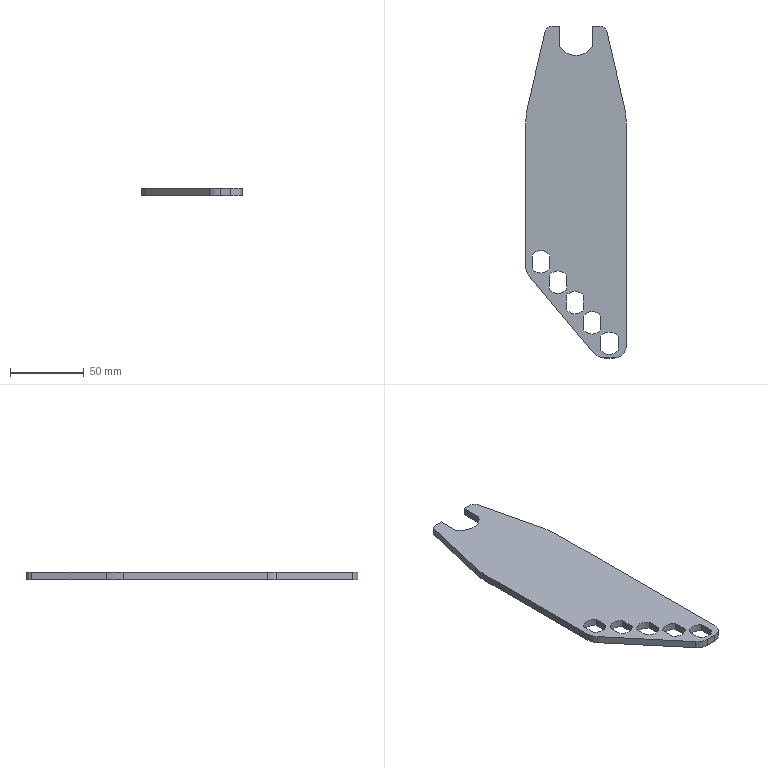Part | SolidWorks | features Fillet 5, ICE 5, Extrusion 1, LPattern 1 | 1 solid | 40 faces | box 68 x 225 x 5 mm | volume 59113 mm3 | plane 22 | cylinder 18 | commonest cylinder face diameters 15.2 x10 10 x2 20 x2 100 x2 16 x1 26 x1
STEP:
#1=CARTESIAN_POINT('',(-29.781,-52.01,5.));
#2=VERTEX_POINT('',#1);
#3=CARTESIAN_POINT('',(-17.781,-52.01,5.));
#4=VERTEX_POINT('',#3);
#5=CARTESIAN_POINT('',(-23.781,-47.345,5.));
#6=DIRECTION('',(0.,0.,1.));
#7=DIRECTION('',(1.,0.,0.));
#8=AXIS2_PLACEMENT_3D('',#5,#6,#7);
#9=CIRCLE('',#8,7.6);
#10=EDGE_CURVE('',#2,#4,#9,.T.);
#11=ORIENTED_EDGE('',*,*,#10,.T.);
#12=CARTESIAN_POINT('',(-17.781,-52.01,0.));
#13=VERTEX_POINT('',#12);
#14=CARTESIAN_POINT('',(-17.781,-52.01,0.));
#15=DIRECTION('',(0.,0.,1.));
#16=VECTOR('',#15,1000.);
#17=LINE('',#14,#16);
#18=EDGE_CURVE('',#13,#4,#17,.T.);
#19=ORIENTED_EDGE('',*,*,#18,.F.);
#20=CARTESIAN_POINT('',(-29.781,-52.01,0.));
#21=VERTEX_POINT('',#20);
#22=CARTESIAN_POINT('',(-23.781,-47.345,0.));
#23=DIRECTION('',(0.,0.,1.));
#24=DIRECTION('',(1.,0.,0.));
#25=AXIS2_PLACEMENT_3D('',#22,#23,#24);
#26=CIRCLE('',#25,7.6);
#27=EDGE_CURVE('',#21,#13,#26,.T.);
#28=ORIENTED_EDGE('',*,*,#27,.F.);
#29=CARTESIAN_POINT('',(-29.781,-52.01,0.));
#30=DIRECTION('',(0.,0.,1.));
#31=VECTOR('',#30,1000.);
#32=LINE('',#29,#31);
#33=EDGE_CURVE('',#21,#2,#32,.T.);
#34=ORIENTED_EDGE('',*,*,#33,.T.);
#35=EDGE_LOOP('',(#11,#19,#28,#34));
#36=FACE_OUTER_BOUND('',#35,.T.);
#37=CARTESIAN_POINT('',(-23.781,-47.345,-3.));
#38=DIRECTION('',(0.,0.,1.));
#39=DIRECTION('',(1.,0.,0.));
#40=AXIS2_PLACEMENT_3D('',#37,#38,#39);
#41=CYLINDRICAL_SURFACE('',#40,7.6);
#42=ADVANCED_FACE('',(#36),#41,.F.);
#43=CARTESIAN_POINT('',(-18.211,-65.798,5.));
#44=VERTEX_POINT('',#43);
#45=CARTESIAN_POINT('',(-6.211,-65.798,5.));
#46=VERTEX_POINT('',#45);
#47=CARTESIAN_POINT('',(-12.211,-61.134,5.));
#48=DIRECTION('',(0.,0.,1.));
#49=DIRECTION('',(1.,0.,0.));
#50=AXIS2_PLACEMENT_3D('',#47,#48,#49);
#51=CIRCLE('',#50,7.6);
#52=EDGE_CURVE('',#44,#46,#51,.T.);
#53=ORIENTED_EDGE('',*,*,#52,.T.);
#54=CARTESIAN_POINT('',(-6.211,-65.798,0.));
#55=VERTEX_POINT('',#54);
#56=CARTESIAN_POINT('',(-6.211,-65.798,0.));
#57=DIRECTION('',(0.,0.,1.));
#58=VECTOR('',#57,1000.);
#59=LINE('',#56,#58);
#60=EDGE_CURVE('',#55,#46,#59,.T.);
#61=ORIENTED_EDGE('',*,*,#60,.F.);
#62=CARTESIAN_POINT('',(-18.211,-65.798,0.));
#63=VERTEX_POINT('',#62);
#64=CARTESIAN_POINT('',(-12.211,-61.134,0.));
#65=DIRECTION('',(0.,0.,1.));
#66=DIRECTION('',(1.,0.,0.));
#67=AXIS2_PLACEMENT_3D('',#64,#65,#66);
#68=CIRCLE('',#67,7.6);
#69=EDGE_CURVE('',#63,#55,#68,.T.);
#70=ORIENTED_EDGE('',*,*,#69,.F.);
#71=CARTESIAN_POINT('',(-18.211,-65.798,0.));
#72=DIRECTION('',(0.,0.,1.));
#73=VECTOR('',#72,1000.);
#74=LINE('',#71,#73);
#75=EDGE_CURVE('',#63,#44,#74,.T.);
#76=ORIENTED_EDGE('',*,*,#75,.T.);
#77=EDGE_LOOP('',(#53,#61,#70,#76));
#78=FACE_OUTER_BOUND('',#77,.T.);
#79=CARTESIAN_POINT('',(-12.211,-61.134,-3.));
#80=DIRECTION('',(0.,0.,1.));
#81=DIRECTION('',(1.,0.,0.));
#82=AXIS2_PLACEMENT_3D('',#79,#80,#81);
#83=CYLINDRICAL_SURFACE('',#82,7.6);
#84=ADVANCED_FACE('',(#78),#83,.F.);
#85=CARTESIAN_POINT('',(-6.64,-79.587,5.));
#86=VERTEX_POINT('',#85);
#87=CARTESIAN_POINT('',(5.36,-79.587,5.));
#88=VERTEX_POINT('',#87);
#89=CARTESIAN_POINT('',(-0.6404,-74.922,5.));
#90=DIRECTION('',(0.,0.,1.));
#91=DIRECTION('',(1.,0.,0.));
#92=AXIS2_PLACEMENT_3D('',#89,#90,#91);
#93=CIRCLE('',#92,7.6);
#94=EDGE_CURVE('',#86,#88,#93,.T.);
#95=ORIENTED_EDGE('',*,*,#94,.T.);
#96=CARTESIAN_POINT('',(5.36,-79.587,0.));
#97=VERTEX_POINT('',#96);
#98=CARTESIAN_POINT('',(5.36,-79.587,0.));
#99=DIRECTION('',(0.,0.,1.));
#100=VECTOR('',#99,1000.);
#101=LINE('',#98,#100);
#102=EDGE_CURVE('',#97,#88,#101,.T.);
#103=ORIENTED_EDGE('',*,*,#102,.F.);
#104=CARTESIAN_POINT('',(-6.64,-79.587,0.));
#105=VERTEX_POINT('',#104);
#106=CARTESIAN_POINT('',(-0.6404,-74.922,0.));
#107=DIRECTION('',(0.,0.,1.));
#108=DIRECTION('',(1.,0.,0.));
#109=AXIS2_PLACEMENT_3D('',#106,#107,#108);
#110=CIRCLE('',#109,7.6);
#111=EDGE_CURVE('',#105,#97,#110,.T.);
#112=ORIENTED_EDGE('',*,*,#111,.F.);
#113=CARTESIAN_POINT('',(-6.64,-79.587,0.));
#114=DIRECTION('',(0.,0.,1.));
#115=VECTOR('',#114,1000.);
#116=LINE('',#113,#115);
#117=EDGE_CURVE('',#105,#86,#116,.T.);
#118=ORIENTED_EDGE('',*,*,#117,.T.);
#119=EDGE_LOOP('',(#95,#103,#112,#118));
#120=FACE_OUTER_BOUND('',#119,.T.);
#121=CARTESIAN_POINT('',(-0.6404,-74.922,-3.));
#122=DIRECTION('',(0.,0.,1.));
#123=DIRECTION('',(1.,0.,0.));
#124=AXIS2_PLACEMENT_3D('',#121,#122,#123);
#125=CYLINDRICAL_SURFACE('',#124,7.6);
#126=ADVANCED_FACE('',(#120),#125,.F.);
#127=CARTESIAN_POINT('',(4.93,-93.376,5.));
#128=VERTEX_POINT('',#127);
#129=CARTESIAN_POINT('',(16.93,-93.376,5.));
#130=VERTEX_POINT('',#129);
#131=CARTESIAN_POINT('',(10.93,-88.711,5.));
#132=DIRECTION('',(0.,0.,1.));
#133=DIRECTION('',(1.,0.,0.));
#134=AXIS2_PLACEMENT_3D('',#131,#132,#133);
#135=CIRCLE('',#134,7.6);
#136=EDGE_CURVE('',#128,#130,#135,.T.);
#137=ORIENTED_EDGE('',*,*,#136,.T.);
#138=CARTESIAN_POINT('',(16.93,-93.376,0.));
#139=VERTEX_POINT('',#138);
#140=CARTESIAN_POINT('',(16.93,-93.376,0.));
#141=DIRECTION('',(0.,0.,1.));
#142=VECTOR('',#141,1000.);
#143=LINE('',#140,#142);
#144=EDGE_CURVE('',#139,#130,#143,.T.);
#145=ORIENTED_EDGE('',*,*,#144,.F.);
#146=CARTESIAN_POINT('',(4.93,-93.376,0.));
#147=VERTEX_POINT('',#146);
#148=CARTESIAN_POINT('',(10.93,-88.711,0.));
#149=DIRECTION('',(0.,0.,1.));
#150=DIRECTION('',(1.,0.,0.));
#151=AXIS2_PLACEMENT_3D('',#148,#149,#150);
#152=CIRCLE('',#151,7.6);
#153=EDGE_CURVE('',#147,#139,#152,.T.);
#154=ORIENTED_EDGE('',*,*,#153,.F.);
#155=CARTESIAN_POINT('',(4.93,-93.376,0.));
#156=DIRECTION('',(0.,0.,1.));
#157=VECTOR('',#156,1000.);
#158=LINE('',#155,#157);
#159=EDGE_CURVE('',#147,#128,#158,.T.);
#160=ORIENTED_EDGE('',*,*,#159,.T.);
#161=EDGE_LOOP('',(#137,#145,#154,#160));
#162=FACE_OUTER_BOUND('',#161,.T.);
#163=CARTESIAN_POINT('',(10.93,-88.711,-3.));
#164=DIRECTION('',(0.,0.,1.));
#165=DIRECTION('',(1.,0.,0.));
#166=AXIS2_PLACEMENT_3D('',#163,#164,#165);
#167=CYLINDRICAL_SURFACE('',#166,7.6);
#168=ADVANCED_FACE('',(#162),#167,.F.);
#169=CARTESIAN_POINT('',(16.5,-107.165,5.));
#170=VERTEX_POINT('',#169);
#171=CARTESIAN_POINT('',(28.5,-107.165,5.));
#172=VERTEX_POINT('',#171);
#173=CARTESIAN_POINT('',(22.5,-102.5,5.));
#174=DIRECTION('',(0.,0.,1.));
#175=DIRECTION('',(1.,0.,0.));
#176=AXIS2_PLACEMENT_3D('',#173,#174,#175);
#177=CIRCLE('',#176,7.6);
#178=EDGE_CURVE('',#170,#172,#177,.T.);
#179=ORIENTED_EDGE('',*,*,#178,.T.);
#180=CARTESIAN_POINT('',(28.5,-107.165,0.));
#181=VERTEX_POINT('',#180);
#182=CARTESIAN_POINT('',(28.5,-107.165,0.));
#183=DIRECTION('',(0.,0.,1.));
#184=VECTOR('',#183,1000.);
#185=LINE('',#182,#184);
#186=EDGE_CURVE('',#181,#172,#185,.T.);
#187=ORIENTED_EDGE('',*,*,#186,.F.);
#188=CARTESIAN_POINT('',(16.5,-107.165,0.));
#189=VERTEX_POINT('',#188);
#190=CARTESIAN_POINT('',(22.5,-102.5,0.));
#191=DIRECTION('',(0.,0.,1.));
#192=DIRECTION('',(1.,0.,0.));
#193=AXIS2_PLACEMENT_3D('',#190,#191,#192);
#194=CIRCLE('',#193,7.6);
#195=EDGE_CURVE('',#189,#181,#194,.T.);
#196=ORIENTED_EDGE('',*,*,#195,.F.);
#197=CARTESIAN_POINT('',(16.5,-107.165,0.));
#198=DIRECTION('',(0.,0.,1.));
#199=VECTOR('',#198,1000.);
#200=LINE('',#197,#199);
#201=EDGE_CURVE('',#189,#170,#200,.T.);
#202=ORIENTED_EDGE('',*,*,#201,.T.);
#203=EDGE_LOOP('',(#179,#187,#196,#202));
#204=FACE_OUTER_BOUND('',#203,.T.);
#205=CARTESIAN_POINT('',(22.5,-102.5,-3.));
#206=DIRECTION('',(0.,0.,1.));
#207=DIRECTION('',(1.,0.,0.));
#208=AXIS2_PLACEMENT_3D('',#205,#206,#207);
#209=CYLINDRICAL_SURFACE('',#208,7.6);
#210=ADVANCED_FACE('',(#204),#209,.F.);
#211=CARTESIAN_POINT('',(16.032,112.5,5.));
#212=VERTEX_POINT('',#211);
#213=CARTESIAN_POINT('',(11.,112.5,5.));
#214=VERTEX_POINT('',#213);
#215=CARTESIAN_POINT('',(-34.,112.5,5.));
#216=DIRECTION('',(-1.,0.,0.));
#217=VECTOR('',#216,1000.);
#218=LINE('',#215,#217);
#219=EDGE_CURVE('',#212,#214,#218,.T.);
#220=ORIENTED_EDGE('',*,*,#219,.F.);
#221=CARTESIAN_POINT('',(16.032,112.5,0.));
#222=VERTEX_POINT('',#221);
#223=CARTESIAN_POINT('',(16.032,112.5,5.));
#224=DIRECTION('',(0.,0.,-1.));
#225=VECTOR('',#224,1000.);
#226=LINE('',#223,#225);
#227=EDGE_CURVE('',#212,#222,#226,.T.);
#228=ORIENTED_EDGE('',*,*,#227,.T.);
#229=CARTESIAN_POINT('',(11.,112.5,0.));
#230=VERTEX_POINT('',#229);
#231=CARTESIAN_POINT('',(-34.,112.5,0.));
#232=DIRECTION('',(-1.,0.,0.));
#233=VECTOR('',#232,1000.);
#234=LINE('',#231,#233);
#235=EDGE_CURVE('',#222,#230,#234,.T.);
#236=ORIENTED_EDGE('',*,*,#235,.T.);
#237=CARTESIAN_POINT('',(11.,112.5,-3.));
#238=DIRECTION('',(0.,0.,1.));
#239=VECTOR('',#238,1000.);
#240=LINE('',#237,#239);
#241=EDGE_CURVE('',#230,#214,#240,.T.);
#242=ORIENTED_EDGE('',*,*,#241,.T.);
#243=EDGE_LOOP('',(#220,#228,#236,#242));
#244=FACE_OUTER_BOUND('',#243,.T.);
#245=CARTESIAN_POINT('',(-34.,112.5,5.));
#246=DIRECTION('',(0.,-1.,0.));
#247=DIRECTION('',(0.,0.,-1.));
#248=AXIS2_PLACEMENT_3D('',#245,#246,#247);
#249=PLANE('',#248);
#250=ADVANCED_FACE('',(#244),#249,.F.);
#251=CARTESIAN_POINT('',(34.,-104.5,0.));
#252=VERTEX_POINT('',#251);
#253=CARTESIAN_POINT('',(34.,46.744,0.));
#254=VERTEX_POINT('',#253);
#255=CARTESIAN_POINT('',(34.,112.5,0.));
#256=DIRECTION('',(0.,1.,0.));
#257=VECTOR('',#256,1000.);
#258=LINE('',#255,#257);
#259=EDGE_CURVE('',#252,#254,#258,.T.);
#260=ORIENTED_EDGE('',*,*,#259,.T.);
#261=CARTESIAN_POINT('',(34.,46.744,5.));
#262=VERTEX_POINT('',#261);
#263=CARTESIAN_POINT('',(34.,46.744,5.));
#264=DIRECTION('',(0.,0.,1.));
#265=VECTOR('',#264,1000.);
#266=LINE('',#263,#265);
#267=EDGE_CURVE('',#254,#262,#266,.T.);
#268=ORIENTED_EDGE('',*,*,#267,.T.);
#269=CARTESIAN_POINT('',(34.,-104.5,5.));
#270=VERTEX_POINT('',#269);
#271=CARTESIAN_POINT('',(34.,112.5,5.));
#272=DIRECTION('',(0.,1.,0.));
#273=VECTOR('',#272,1000.);
#274=LINE('',#271,#273);
#275=EDGE_CURVE('',#270,#262,#274,.T.);
#276=ORIENTED_EDGE('',*,*,#275,.F.);
#277=CARTESIAN_POINT('',(34.,-104.5,5.));
#278=DIRECTION('',(0.,0.,-1.));
#279=VECTOR('',#278,1000.);
#280=LINE('',#277,#279);
#281=EDGE_CURVE('',#270,#252,#280,.T.);
#282=ORIENTED_EDGE('',*,*,#281,.T.);
#283=EDGE_LOOP('',(#260,#268,#276,#282));
#284=FACE_OUTER_BOUND('',#283,.T.);
#285=CARTESIAN_POINT('',(34.,112.5,5.));
#286=DIRECTION('',(-1.,0.,0.));
#287=DIRECTION('',(0.,-1.,0.));
#288=AXIS2_PLACEMENT_3D('',#285,#286,#287);
#289=PLANE('',#288);
#290=ADVANCED_FACE('',(#284),#289,.F.);
#291=CARTESIAN_POINT('',(-11.,112.5,0.));
#292=VERTEX_POINT('',#291);
#293=CARTESIAN_POINT('',(-16.032,112.5,0.));
#294=VERTEX_POINT('',#293);
#295=CARTESIAN_POINT('',(-34.,112.5,0.));
#296=DIRECTION('',(-1.,0.,0.));
#297=VECTOR('',#296,1000.);
#298=LINE('',#295,#297);
#299=EDGE_CURVE('',#292,#294,#298,.T.);
#300=ORIENTED_EDGE('',*,*,#299,.T.);
#301=CARTESIAN_POINT('',(-16.032,112.5,5.));
#302=VERTEX_POINT('',#301);
#303=CARTESIAN_POINT('',(-16.032,112.5,5.));
#304=DIRECTION('',(0.,0.,1.));
#305=VECTOR('',#304,1000.);
#306=LINE('',#303,#305);
#307=EDGE_CURVE('',#294,#302,#306,.T.);
#308=ORIENTED_EDGE('',*,*,#307,.T.);
#309=CARTESIAN_POINT('',(-11.,112.5,5.));
#310=VERTEX_POINT('',#309);
#311=CARTESIAN_POINT('',(-34.,112.5,5.));
#312=DIRECTION('',(-1.,0.,0.));
#313=VECTOR('',#312,1000.);
#314=LINE('',#311,#313);
#315=EDGE_CURVE('',#310,#302,#314,.T.);
#316=ORIENTED_EDGE('',*,*,#315,.F.);
#317=CARTESIAN_POINT('',(-11.,112.5,-3.));
#318=DIRECTION('',(0.,0.,1.));
#319=VECTOR('',#318,1000.);
#320=LINE('',#317,#319);
#321=EDGE_CURVE('',#292,#310,#320,.T.);
#322=ORIENTED_EDGE('',*,*,#321,.F.);
#323=EDGE_LOOP('',(#300,#308,#316,#322));
#324=FACE_OUTER_BOUND('',#323,.T.);
#325=CARTESIAN_POINT('',(-34.,112.5,5.));
#326=DIRECTION('',(0.,-1.,0.));
#327=DIRECTION('',(0.,0.,-1.));
#328=AXIS2_PLACEMENT_3D('',#325,#326,#327);
#329=PLANE('',#328);
#330=ADVANCED_FACE('',(#324),#329,.F.);
#331=CARTESIAN_POINT('',(-34.,46.744,5.));
#332=VERTEX_POINT('',#331);
#333=CARTESIAN_POINT('',(-34.,-50.973,5.));
#334=VERTEX_POINT('',#333);
#335=CARTESIAN_POINT('',(-34.,112.5,5.));
#336=DIRECTION('',(0.,-1.,0.));
#337=VECTOR('',#336,1000.);
#338=LINE('',#335,#337);
#339=EDGE_CURVE('',#332,#334,#338,.T.);
#340=ORIENTED_EDGE('',*,*,#339,.F.);
#341=CARTESIAN_POINT('',(-34.,46.744,0.));
#342=VERTEX_POINT('',#341);
#343=CARTESIAN_POINT('',(-34.,46.744,5.));
#344=DIRECTION('',(0.,0.,-1.));
#345=VECTOR('',#344,1000.);
#346=LINE('',#343,#345);
#347=EDGE_CURVE('',#332,#342,#346,.T.);
#348=ORIENTED_EDGE('',*,*,#347,.T.);
#349=CARTESIAN_POINT('',(-34.,-50.973,0.));
#350=VERTEX_POINT('',#349);
#351=CARTESIAN_POINT('',(-34.,112.5,0.));
#352=DIRECTION('',(0.,-1.,0.));
#353=VECTOR('',#352,1000.);
#354=LINE('',#351,#353);
#355=EDGE_CURVE('',#342,#350,#354,.T.);
#356=ORIENTED_EDGE('',*,*,#355,.T.);
#357=CARTESIAN_POINT('',(-34.,-50.973,5.));
#358=DIRECTION('',(0.,0.,1.));
#359=VECTOR('',#358,1000.);
#360=LINE('',#357,#359);
#361=EDGE_CURVE('',#350,#334,#360,.T.);
#362=ORIENTED_EDGE('',*,*,#361,.T.);
#363=EDGE_LOOP('',(#340,#348,#356,#362));
#364=FACE_OUTER_BOUND('',#363,.T.);
#365=CARTESIAN_POINT('',(-34.,112.5,5.));
#366=DIRECTION('',(1.,0.,0.));
#367=DIRECTION('',(0.,1.,0.));
#368=AXIS2_PLACEMENT_3D('',#365,#366,#367);
#369=PLANE('',#368);
#370=ADVANCED_FACE('',(#364),#369,.F.);
#371=CARTESIAN_POINT('',(19.236,-112.5,5.));
#372=VERTEX_POINT('',#371);
#373=CARTESIAN_POINT('',(26.,-112.5,5.));
#374=VERTEX_POINT('',#373);
#375=CARTESIAN_POINT('',(-34.,-112.5,5.));
#376=DIRECTION('',(1.,0.,0.));
#377=VECTOR('',#376,1000.);
#378=LINE('',#375,#377);
#379=EDGE_CURVE('',#372,#374,#378,.T.);
#380=ORIENTED_EDGE('',*,*,#379,.F.);
#381=CARTESIAN_POINT('',(19.236,-112.5,0.));
#382=VERTEX_POINT('',#381);
#383=CARTESIAN_POINT('',(19.236,-112.5,5.));
#384=DIRECTION('',(0.,0.,-1.));
#385=VECTOR('',#384,1000.);
#386=LINE('',#383,#385);
#387=EDGE_CURVE('',#372,#382,#386,.T.);
#388=ORIENTED_EDGE('',*,*,#387,.T.);
#389=CARTESIAN_POINT('',(26.,-112.5,0.));
#390=VERTEX_POINT('',#389);
#391=CARTESIAN_POINT('',(-34.,-112.5,0.));
#392=DIRECTION('',(1.,0.,0.));
#393=VECTOR('',#392,1000.);
#394=LINE('',#391,#393);
#395=EDGE_CURVE('',#382,#390,#394,.T.);
#396=ORIENTED_EDGE('',*,*,#395,.T.);
#397=CARTESIAN_POINT('',(26.,-112.5,5.));
#398=DIRECTION('',(0.,0.,1.));
#399=VECTOR('',#398,1000.);
#400=LINE('',#397,#399);
#401=EDGE_CURVE('',#390,#374,#400,.T.);
#402=ORIENTED_EDGE('',*,*,#401,.T.);
#403=EDGE_LOOP('',(#380,#388,#396,#402));
#404=FACE_OUTER_BOUND('',#403,.T.);
#405=CARTESIAN_POINT('',(-34.,-112.5,5.));
#406=DIRECTION('',(0.,1.,0.));
#407=DIRECTION('',(0.,0.,1.));
#408=AXIS2_PLACEMENT_3D('',#405,#406,#407);
#409=PLANE('',#408);
#410=ADVANCED_FACE('',(#404),#409,.F.);
#411=ORIENTED_EDGE('',*,*,#275,.T.);
#412=CARTESIAN_POINT('',(32.692,58.105,5.));
#413=VERTEX_POINT('',#412);
#414=CARTESIAN_POINT('',(-16.,46.744,5.));
#415=DIRECTION('',(0.,0.,1.));
#416=DIRECTION('',(1.,0.,0.));
#417=AXIS2_PLACEMENT_3D('',#414,#415,#416);
#418=CIRCLE('',#417,50.);
#419=EDGE_CURVE('',#262,#413,#418,.T.);
#420=ORIENTED_EDGE('',*,*,#419,.T.);
#421=CARTESIAN_POINT('',(20.902,108.636,5.));
#422=VERTEX_POINT('',#421);
#423=CARTESIAN_POINT('',(20.,112.5,5.));
#424=DIRECTION('',(0.2272,-0.9738,0.));
#425=VECTOR('',#424,1000.);
#426=LINE('',#423,#425);
#427=EDGE_CURVE('',#422,#413,#426,.T.);
#428=ORIENTED_EDGE('',*,*,#427,.F.);
#429=CARTESIAN_POINT('',(16.032,107.5,5.));
#430=DIRECTION('',(0.,0.,1.));
#431=DIRECTION('',(1.,0.,0.));
#432=AXIS2_PLACEMENT_3D('',#429,#430,#431);
#433=CIRCLE('',#432,5.);
#434=EDGE_CURVE('',#422,#212,#433,.T.);
#435=ORIENTED_EDGE('',*,*,#434,.T.);
#436=ORIENTED_EDGE('',*,*,#219,.T.);
#437=CARTESIAN_POINT('',(11.,98.644,5.));
#438=VERTEX_POINT('',#437);
#439=CARTESIAN_POINT('',(11.,112.5,5.));
#440=DIRECTION('',(0.,1.,0.));
#441=VECTOR('',#440,1000.);
#442=LINE('',#439,#441);
#443=EDGE_CURVE('',#438,#214,#442,.T.);
#444=ORIENTED_EDGE('',*,*,#443,.F.);
#445=CARTESIAN_POINT('',(-11.,98.644,5.));
#446=VERTEX_POINT('',#445);
#447=CARTESIAN_POINT('',(0.,105.572,5.));
#448=DIRECTION('',(0.,0.,1.));
#449=DIRECTION('',(1.,0.,0.));
#450=AXIS2_PLACEMENT_3D('',#447,#448,#449);
#451=CIRCLE('',#450,13.);
#452=EDGE_CURVE('',#446,#438,#451,.T.);
#453=ORIENTED_EDGE('',*,*,#452,.F.);
#454=CARTESIAN_POINT('',(-11.,112.5,5.));
#455=DIRECTION('',(0.,-1.,0.));
#456=VECTOR('',#455,1000.);
#457=LINE('',#454,#456);
#458=EDGE_CURVE('',#310,#446,#457,.T.);
#459=ORIENTED_EDGE('',*,*,#458,.F.);
#460=ORIENTED_EDGE('',*,*,#315,.T.);
#461=CARTESIAN_POINT('',(-20.902,108.636,5.));
#462=VERTEX_POINT('',#461);
#463=CARTESIAN_POINT('',(-16.032,107.5,5.));
#464=DIRECTION('',(0.,0.,1.));
#465=DIRECTION('',(1.,0.,0.));
#466=AXIS2_PLACEMENT_3D('',#463,#464,#465);
#467=CIRCLE('',#466,5.);
#468=EDGE_CURVE('',#302,#462,#467,.T.);
#469=ORIENTED_EDGE('',*,*,#468,.T.);
#470=CARTESIAN_POINT('',(-32.692,58.105,5.));
#471=VERTEX_POINT('',#470);
#472=CARTESIAN_POINT('',(-20.,112.5,5.));
#473=DIRECTION('',(0.2272,0.9738,0.));
#474=VECTOR('',#473,1000.);
#475=LINE('',#472,#474);
#476=EDGE_CURVE('',#471,#462,#475,.T.);
#477=ORIENTED_EDGE('',*,*,#476,.F.);
#478=CARTESIAN_POINT('',(16.,46.744,5.));
#479=DIRECTION('',(0.,0.,1.));
#480=DIRECTION('',(1.,0.,0.));
#481=AXIS2_PLACEMENT_3D('',#478,#479,#480);
#482=CIRCLE('',#481,50.);
#483=EDGE_CURVE('',#471,#332,#482,.T.);
#484=ORIENTED_EDGE('',*,*,#483,.T.);
#485=ORIENTED_EDGE('',*,*,#339,.T.);
#486=CARTESIAN_POINT('',(-31.66,-57.401,5.));
#487=VERTEX_POINT('',#486);
#488=CARTESIAN_POINT('',(-24.,-50.973,5.));
#489=DIRECTION('',(0.,0.,1.));
#490=DIRECTION('',(1.,0.,0.));
#491=AXIS2_PLACEMENT_3D('',#488,#489,#490);
#492=CIRCLE('',#491,10.);
#493=EDGE_CURVE('',#334,#487,#492,.T.);
#494=ORIENTED_EDGE('',*,*,#493,.T.);
#495=CARTESIAN_POINT('',(11.576,-108.928,5.));
#496=VERTEX_POINT('',#495);
#497=CARTESIAN_POINT('',(14.573,-112.5,5.));
#498=DIRECTION('',(-0.6428,0.766,0.));
#499=VECTOR('',#498,1000.);
#500=LINE('',#497,#499);
#501=EDGE_CURVE('',#496,#487,#500,.T.);
#502=ORIENTED_EDGE('',*,*,#501,.F.);
#503=CARTESIAN_POINT('',(19.236,-102.5,5.));
#504=DIRECTION('',(0.,0.,1.));
#505=DIRECTION('',(1.,0.,0.));
#506=AXIS2_PLACEMENT_3D('',#503,#504,#505);
#507=CIRCLE('',#506,10.);
#508=EDGE_CURVE('',#496,#372,#507,.T.);
#509=ORIENTED_EDGE('',*,*,#508,.T.);
#510=ORIENTED_EDGE('',*,*,#379,.T.);
#511=CARTESIAN_POINT('',(26.,-104.5,5.));
#512=DIRECTION('',(0.,0.,1.));
#513=DIRECTION('',(1.,0.,0.));
#514=AXIS2_PLACEMENT_3D('',#511,#512,#513);
#515=CIRCLE('',#514,8.);
#516=EDGE_CURVE('',#374,#270,#515,.T.);
#517=ORIENTED_EDGE('',*,*,#516,.T.);
#518=EDGE_LOOP('',(#411,#420,#428,#435,#436,#444,#453,#459,#460,#469,#477,#484,#485,#494,#502,#509,#510,#517));
#519=FACE_OUTER_BOUND('',#518,.T.);
#520=ORIENTED_EDGE('',*,*,#94,.F.);
#521=CARTESIAN_POINT('',(-6.64,-70.258,5.));
#522=VERTEX_POINT('',#521);
#523=CARTESIAN_POINT('',(-6.64,-79.587,5.));
#524=DIRECTION('',(0.,1.,0.));
#525=VECTOR('',#524,1000.);
#526=LINE('',#523,#525);
#527=EDGE_CURVE('',#86,#522,#526,.T.);
#528=ORIENTED_EDGE('',*,*,#527,.T.);
#529=CARTESIAN_POINT('',(5.36,-70.258,5.));
#530=VERTEX_POINT('',#529);
#531=CARTESIAN_POINT('',(-0.6404,-74.922,5.));
#532=DIRECTION('',(0.,0.,1.));
#533=DIRECTION('',(1.,0.,0.));
#534=AXIS2_PLACEMENT_3D('',#531,#532,#533);
#535=CIRCLE('',#534,7.6);
#536=EDGE_CURVE('',#530,#522,#535,.T.);
#537=ORIENTED_EDGE('',*,*,#536,.F.);
#538=CARTESIAN_POINT('',(5.36,-79.587,5.));
#539=DIRECTION('',(0.,-1.,0.));
#540=VECTOR('',#539,1000.);
#541=LINE('',#538,#540);
#542=EDGE_CURVE('',#530,#88,#541,.T.);
#543=ORIENTED_EDGE('',*,*,#542,.T.);
#544=EDGE_LOOP('',(#520,#528,#537,#543));
#545=FACE_BOUND('',#544,.T.);
#546=ORIENTED_EDGE('',*,*,#136,.F.);
#547=CARTESIAN_POINT('',(4.93,-84.046,5.));
#548=VERTEX_POINT('',#547);
#549=CARTESIAN_POINT('',(4.93,-93.376,5.));
#550=DIRECTION('',(0.,1.,0.));
#551=VECTOR('',#550,1000.);
#552=LINE('',#549,#551);
#553=EDGE_CURVE('',#128,#548,#552,.T.);
#554=ORIENTED_EDGE('',*,*,#553,.T.);
#555=CARTESIAN_POINT('',(16.93,-84.046,5.));
#556=VERTEX_POINT('',#555);
#557=CARTESIAN_POINT('',(10.93,-88.711,5.));
#558=DIRECTION('',(0.,0.,1.));
#559=DIRECTION('',(1.,0.,0.));
#560=AXIS2_PLACEMENT_3D('',#557,#558,#559);
#561=CIRCLE('',#560,7.6);
#562=EDGE_CURVE('',#556,#548,#561,.T.);
#563=ORIENTED_EDGE('',*,*,#562,.F.);
#564=CARTESIAN_POINT('',(16.93,-93.376,5.));
#565=DIRECTION('',(0.,-1.,0.));
#566=VECTOR('',#565,1000.);
#567=LINE('',#564,#566);
#568=EDGE_CURVE('',#556,#130,#567,.T.);
#569=ORIENTED_EDGE('',*,*,#568,.T.);
#570=EDGE_LOOP('',(#546,#554,#563,#569));
#571=FACE_BOUND('',#570,.T.);
#572=ORIENTED_EDGE('',*,*,#10,.F.);
#573=CARTESIAN_POINT('',(-29.781,-42.68,5.));
#574=VERTEX_POINT('',#573);
#575=CARTESIAN_POINT('',(-29.781,-52.01,5.));
#576=DIRECTION('',(0.,1.,0.));
#577=VECTOR('',#576,1000.);
#578=LINE('',#575,#577);
#579=EDGE_CURVE('',#2,#574,#578,.T.);
#580=ORIENTED_EDGE('',*,*,#579,.T.);
#581=CARTESIAN_POINT('',(-17.781,-42.68,5.));
#582=VERTEX_POINT('',#581);
#583=CARTESIAN_POINT('',(-23.781,-47.345,5.));
#584=DIRECTION('',(0.,0.,1.));
#585=DIRECTION('',(1.,0.,0.));
#586=AXIS2_PLACEMENT_3D('',#583,#584,#585);
#587=CIRCLE('',#586,7.6);
#588=EDGE_CURVE('',#582,#574,#587,.T.);
#589=ORIENTED_EDGE('',*,*,#588,.F.);
#590=CARTESIAN_POINT('',(-17.781,-52.01,5.));
#591=DIRECTION('',(0.,-1.,0.));
#592=VECTOR('',#591,1000.);
#593=LINE('',#590,#592);
#594=EDGE_CURVE('',#582,#4,#593,.T.);
#595=ORIENTED_EDGE('',*,*,#594,.T.);
#596=EDGE_LOOP('',(#572,#580,#589,#595));
#597=FACE_BOUND('',#596,.T.);
#598=ORIENTED_EDGE('',*,*,#52,.F.);
#599=CARTESIAN_POINT('',(-18.211,-56.469,5.));
#600=VERTEX_POINT('',#599);
#601=CARTESIAN_POINT('',(-18.211,-65.798,5.));
#602=DIRECTION('',(0.,1.,0.));
#603=VECTOR('',#602,1000.);
#604=LINE('',#601,#603);
#605=EDGE_CURVE('',#44,#600,#604,.T.);
#606=ORIENTED_EDGE('',*,*,#605,.T.);
#607=CARTESIAN_POINT('',(-6.211,-56.469,5.));
#608=VERTEX_POINT('',#607);
#609=CARTESIAN_POINT('',(-12.211,-61.134,5.));
#610=DIRECTION('',(0.,0.,1.));
#611=DIRECTION('',(1.,0.,0.));
#612=AXIS2_PLACEMENT_3D('',#609,#610,#611);
#613=CIRCLE('',#612,7.6);
#614=EDGE_CURVE('',#608,#600,#613,.T.);
#615=ORIENTED_EDGE('',*,*,#614,.F.);
#616=CARTESIAN_POINT('',(-6.211,-65.798,5.));
#617=DIRECTION('',(0.,-1.,0.));
#618=VECTOR('',#617,1000.);
#619=LINE('',#616,#618);
#620=EDGE_CURVE('',#608,#46,#619,.T.);
#621=ORIENTED_EDGE('',*,*,#620,.T.);
#622=EDGE_LOOP('',(#598,#606,#615,#621));
#623=FACE_BOUND('',#622,.T.);
#624=ORIENTED_EDGE('',*,*,#178,.F.);
#625=CARTESIAN_POINT('',(16.5,-97.835,5.));
#626=VERTEX_POINT('',#625);
#627=CARTESIAN_POINT('',(16.5,-107.165,5.));
#628=DIRECTION('',(0.,1.,0.));
#629=VECTOR('',#628,1000.);
#630=LINE('',#627,#629);
#631=EDGE_CURVE('',#170,#626,#630,.T.);
#632=ORIENTED_EDGE('',*,*,#631,.T.);
#633=CARTESIAN_POINT('',(28.5,-97.835,5.));
#634=VERTEX_POINT('',#633);
#635=CARTESIAN_POINT('',(22.5,-102.5,5.));
#636=DIRECTION('',(0.,0.,1.));
#637=DIRECTION('',(1.,0.,0.));
#638=AXIS2_PLACEMENT_3D('',#635,#636,#637);
#639=CIRCLE('',#638,7.6);
#640=EDGE_CURVE('',#634,#626,#639,.T.);
#641=ORIENTED_EDGE('',*,*,#640,.F.);
#642=CARTESIAN_POINT('',(28.5,-107.165,5.));
#643=DIRECTION('',(0.,-1.,0.));
#644=VECTOR('',#643,1000.);
#645=LINE('',#642,#644);
#646=EDGE_CURVE('',#634,#172,#645,.T.);
#647=ORIENTED_EDGE('',*,*,#646,.T.);
#648=EDGE_LOOP('',(#624,#632,#641,#647));
#649=FACE_BOUND('',#648,.T.);
#650=CARTESIAN_POINT('',(0.,0.,5.));
#651=DIRECTION('',(0.,0.,1.));
#652=DIRECTION('',(1.,0.,0.));
#653=AXIS2_PLACEMENT_3D('',#650,#651,#652);
#654=PLANE('',#653);
#655=ADVANCED_FACE('',(#519,#545,#571,#597,#623,#649),#654,.T.);
#656=ORIENTED_EDGE('',*,*,#111,.T.);
#657=CARTESIAN_POINT('',(5.36,-70.258,0.));
#658=VERTEX_POINT('',#657);
#659=CARTESIAN_POINT('',(5.36,-79.587,0.));
#660=DIRECTION('',(0.,-1.,0.));
#661=VECTOR('',#660,1000.);
#662=LINE('',#659,#661);
#663=EDGE_CURVE('',#658,#97,#662,.T.);
#664=ORIENTED_EDGE('',*,*,#663,.F.);
#665=CARTESIAN_POINT('',(-6.64,-70.258,0.));
#666=VERTEX_POINT('',#665);
#667=CARTESIAN_POINT('',(-0.6404,-74.922,0.));
#668=DIRECTION('',(0.,0.,1.));
#669=DIRECTION('',(1.,0.,0.));
#670=AXIS2_PLACEMENT_3D('',#667,#668,#669);
#671=CIRCLE('',#670,7.6);
#672=EDGE_CURVE('',#658,#666,#671,.T.);
#673=ORIENTED_EDGE('',*,*,#672,.T.);
#674=CARTESIAN_POINT('',(-6.64,-79.587,0.));
#675=DIRECTION('',(0.,1.,0.));
#676=VECTOR('',#675,1000.);
#677=LINE('',#674,#676);
#678=EDGE_CURVE('',#105,#666,#677,.T.);
#679=ORIENTED_EDGE('',*,*,#678,.F.);
#680=EDGE_LOOP('',(#656,#664,#673,#679));
#681=FACE_BOUND('',#680,.T.);
#682=ORIENTED_EDGE('',*,*,#153,.T.);
#683=CARTESIAN_POINT('',(16.93,-84.046,0.));
#684=VERTEX_POINT('',#683);
#685=CARTESIAN_POINT('',(16.93,-93.376,0.));
#686=DIRECTION('',(0.,-1.,0.));
#687=VECTOR('',#686,1000.);
#688=LINE('',#685,#687);
#689=EDGE_CURVE('',#684,#139,#688,.T.);
#690=ORIENTED_EDGE('',*,*,#689,.F.);
#691=CARTESIAN_POINT('',(4.93,-84.046,0.));
#692=VERTEX_POINT('',#691);
#693=CARTESIAN_POINT('',(10.93,-88.711,0.));
#694=DIRECTION('',(0.,0.,1.));
#695=DIRECTION('',(1.,0.,0.));
#696=AXIS2_PLACEMENT_3D('',#693,#694,#695);
#697=CIRCLE('',#696,7.6);
#698=EDGE_CURVE('',#684,#692,#697,.T.);
#699=ORIENTED_EDGE('',*,*,#698,.T.);
#700=CARTESIAN_POINT('',(4.93,-93.376,0.));
#701=DIRECTION('',(0.,1.,0.));
#702=VECTOR('',#701,1000.);
#703=LINE('',#700,#702);
#704=EDGE_CURVE('',#147,#692,#703,.T.);
#705=ORIENTED_EDGE('',*,*,#704,.F.);
#706=EDGE_LOOP('',(#682,#690,#699,#705));
#707=FACE_BOUND('',#706,.T.);
#708=ORIENTED_EDGE('',*,*,#27,.T.);
#709=CARTESIAN_POINT('',(-17.781,-42.68,0.));
#710=VERTEX_POINT('',#709);
#711=CARTESIAN_POINT('',(-17.781,-52.01,0.));
#712=DIRECTION('',(0.,-1.,0.));
#713=VECTOR('',#712,1000.);
#714=LINE('',#711,#713);
#715=EDGE_CURVE('',#710,#13,#714,.T.);
#716=ORIENTED_EDGE('',*,*,#715,.F.);
#717=CARTESIAN_POINT('',(-29.781,-42.68,0.));
#718=VERTEX_POINT('',#717);
#719=CARTESIAN_POINT('',(-23.781,-47.345,0.));
#720=DIRECTION('',(0.,0.,1.));
#721=DIRECTION('',(1.,0.,0.));
#722=AXIS2_PLACEMENT_3D('',#719,#720,#721);
#723=CIRCLE('',#722,7.6);
#724=EDGE_CURVE('',#710,#718,#723,.T.);
#725=ORIENTED_EDGE('',*,*,#724,.T.);
#726=CARTESIAN_POINT('',(-29.781,-52.01,0.));
#727=DIRECTION('',(0.,1.,0.));
#728=VECTOR('',#727,1000.);
#729=LINE('',#726,#728);
#730=EDGE_CURVE('',#21,#718,#729,.T.);
#731=ORIENTED_EDGE('',*,*,#730,.F.);
#732=EDGE_LOOP('',(#708,#716,#725,#731));
#733=FACE_BOUND('',#732,.T.);
#734=ORIENTED_EDGE('',*,*,#69,.T.);
#735=CARTESIAN_POINT('',(-6.211,-56.469,0.));
#736=VERTEX_POINT('',#735);
#737=CARTESIAN_POINT('',(-6.211,-65.798,0.));
#738=DIRECTION('',(0.,-1.,0.));
#739=VECTOR('',#738,1000.);
#740=LINE('',#737,#739);
#741=EDGE_CURVE('',#736,#55,#740,.T.);
#742=ORIENTED_EDGE('',*,*,#741,.F.);
#743=CARTESIAN_POINT('',(-18.211,-56.469,0.));
#744=VERTEX_POINT('',#743);
#745=CARTESIAN_POINT('',(-12.211,-61.134,0.));
#746=DIRECTION('',(0.,0.,1.));
#747=DIRECTION('',(1.,0.,0.));
#748=AXIS2_PLACEMENT_3D('',#745,#746,#747);
#749=CIRCLE('',#748,7.6);
#750=EDGE_CURVE('',#736,#744,#749,.T.);
#751=ORIENTED_EDGE('',*,*,#750,.T.);
#752=CARTESIAN_POINT('',(-18.211,-65.798,0.));
#753=DIRECTION('',(0.,1.,0.));
#754=VECTOR('',#753,1000.);
#755=LINE('',#752,#754);
#756=EDGE_CURVE('',#63,#744,#755,.T.);
#757=ORIENTED_EDGE('',*,*,#756,.F.);
#758=EDGE_LOOP('',(#734,#742,#751,#757));
#759=FACE_BOUND('',#758,.T.);
#760=ORIENTED_EDGE('',*,*,#195,.T.);
#761=CARTESIAN_POINT('',(28.5,-97.835,0.));
#762=VERTEX_POINT('',#761);
#763=CARTESIAN_POINT('',(28.5,-107.165,0.));
#764=DIRECTION('',(0.,-1.,0.));
#765=VECTOR('',#764,1000.);
#766=LINE('',#763,#765);
#767=EDGE_CURVE('',#762,#181,#766,.T.);
#768=ORIENTED_EDGE('',*,*,#767,.F.);
#769=CARTESIAN_POINT('',(16.5,-97.835,0.));
#770=VERTEX_POINT('',#769);
#771=CARTESIAN_POINT('',(22.5,-102.5,0.));
#772=DIRECTION('',(0.,0.,1.));
#773=DIRECTION('',(1.,0.,0.));
#774=AXIS2_PLACEMENT_3D('',#771,#772,#773);
#775=CIRCLE('',#774,7.6);
#776=EDGE_CURVE('',#762,#770,#775,.T.);
#777=ORIENTED_EDGE('',*,*,#776,.T.);
#778=CARTESIAN_POINT('',(16.5,-107.165,0.));
#779=DIRECTION('',(0.,1.,0.));
#780=VECTOR('',#779,1000.);
#781=LINE('',#778,#780);
#782=EDGE_CURVE('',#189,#770,#781,.T.);
#783=ORIENTED_EDGE('',*,*,#782,.F.);
#784=EDGE_LOOP('',(#760,#768,#777,#783));
#785=FACE_BOUND('',#784,.T.);
#786=CARTESIAN_POINT('',(20.902,108.636,0.));
#787=VERTEX_POINT('',#786);
#788=CARTESIAN_POINT('',(32.692,58.105,0.));
#789=VERTEX_POINT('',#788);
#790=CARTESIAN_POINT('',(20.,112.5,0.));
#791=DIRECTION('',(0.2272,-0.9738,0.));
#792=VECTOR('',#791,1000.);
#793=LINE('',#790,#792);
#794=EDGE_CURVE('',#787,#789,#793,.T.);
#795=ORIENTED_EDGE('',*,*,#794,.T.);
#796=CARTESIAN_POINT('',(-16.,46.744,0.));
#797=DIRECTION('',(0.,0.,-1.));
#798=DIRECTION('',(1.,0.,0.));
#799=AXIS2_PLACEMENT_3D('',#796,#797,#798);
#800=CIRCLE('',#799,50.);
#801=EDGE_CURVE('',#789,#254,#800,.T.);
#802=ORIENTED_EDGE('',*,*,#801,.T.);
#803=ORIENTED_EDGE('',*,*,#259,.F.);
#804=CARTESIAN_POINT('',(26.,-104.5,0.));
#805=DIRECTION('',(0.,0.,-1.));
#806=DIRECTION('',(1.,0.,0.));
#807=AXIS2_PLACEMENT_3D('',#804,#805,#806);
#808=CIRCLE('',#807,8.);
#809=EDGE_CURVE('',#252,#390,#808,.T.);
#810=ORIENTED_EDGE('',*,*,#809,.T.);
#811=ORIENTED_EDGE('',*,*,#395,.F.);
#812=CARTESIAN_POINT('',(11.576,-108.928,0.));
#813=VERTEX_POINT('',#812);
#814=CARTESIAN_POINT('',(19.236,-102.5,0.));
#815=DIRECTION('',(0.,0.,-1.));
#816=DIRECTION('',(1.,0.,0.));
#817=AXIS2_PLACEMENT_3D('',#814,#815,#816);
#818=CIRCLE('',#817,10.);
#819=EDGE_CURVE('',#382,#813,#818,.T.);
#820=ORIENTED_EDGE('',*,*,#819,.T.);
#821=CARTESIAN_POINT('',(-31.66,-57.401,0.));
#822=VERTEX_POINT('',#821);
#823=CARTESIAN_POINT('',(14.573,-112.5,0.));
#824=DIRECTION('',(-0.6428,0.766,0.));
#825=VECTOR('',#824,1000.);
#826=LINE('',#823,#825);
#827=EDGE_CURVE('',#813,#822,#826,.T.);
#828=ORIENTED_EDGE('',*,*,#827,.T.);
#829=CARTESIAN_POINT('',(-24.,-50.973,0.));
#830=DIRECTION('',(0.,0.,-1.));
#831=DIRECTION('',(1.,0.,0.));
#832=AXIS2_PLACEMENT_3D('',#829,#830,#831);
#833=CIRCLE('',#832,10.);
#834=EDGE_CURVE('',#822,#350,#833,.T.);
#835=ORIENTED_EDGE('',*,*,#834,.T.);
#836=ORIENTED_EDGE('',*,*,#355,.F.);
#837=CARTESIAN_POINT('',(-32.692,58.105,0.));
#838=VERTEX_POINT('',#837);
#839=CARTESIAN_POINT('',(16.,46.744,0.));
#840=DIRECTION('',(0.,0.,-1.));
#841=DIRECTION('',(1.,0.,0.));
#842=AXIS2_PLACEMENT_3D('',#839,#840,#841);
#843=CIRCLE('',#842,50.);
#844=EDGE_CURVE('',#342,#838,#843,.T.);
#845=ORIENTED_EDGE('',*,*,#844,.T.);
#846=CARTESIAN_POINT('',(-20.902,108.636,0.));
#847=VERTEX_POINT('',#846);
#848=CARTESIAN_POINT('',(-20.,112.5,0.));
#849=DIRECTION('',(0.2272,0.9738,0.));
#850=VECTOR('',#849,1000.);
#851=LINE('',#848,#850);
#852=EDGE_CURVE('',#838,#847,#851,.T.);
#853=ORIENTED_EDGE('',*,*,#852,.T.);
#854=CARTESIAN_POINT('',(-16.032,107.5,0.));
#855=DIRECTION('',(0.,0.,-1.));
#856=DIRECTION('',(1.,0.,0.));
#857=AXIS2_PLACEMENT_3D('',#854,#855,#856);
#858=CIRCLE('',#857,5.);
#859=EDGE_CURVE('',#847,#294,#858,.T.);
#860=ORIENTED_EDGE('',*,*,#859,.T.);
#861=ORIENTED_EDGE('',*,*,#299,.F.);
#862=CARTESIAN_POINT('',(-11.,98.644,0.));
#863=VERTEX_POINT('',#862);
#864=CARTESIAN_POINT('',(-11.,0.,0.));
#865=DIRECTION('',(0.,-1.,0.));
#866=VECTOR('',#865,1000.);
#867=LINE('',#864,#866);
#868=EDGE_CURVE('',#292,#863,#867,.T.);
#869=ORIENTED_EDGE('',*,*,#868,.T.);
#870=CARTESIAN_POINT('',(11.,98.644,0.));
#871=VERTEX_POINT('',#870);
#872=CARTESIAN_POINT('',(0.,105.572,0.));
#873=DIRECTION('',(0.,0.,1.));
#874=DIRECTION('',(1.,0.,0.));
#875=AXIS2_PLACEMENT_3D('',#872,#873,#874);
#876=CIRCLE('',#875,13.);
#877=EDGE_CURVE('',#863,#871,#876,.T.);
#878=ORIENTED_EDGE('',*,*,#877,.T.);
#879=CARTESIAN_POINT('',(11.,0.,0.));
#880=DIRECTION('',(0.,1.,0.));
#881=VECTOR('',#880,1000.);
#882=LINE('',#879,#881);
#883=EDGE_CURVE('',#871,#230,#882,.T.);
#884=ORIENTED_EDGE('',*,*,#883,.T.);
#885=ORIENTED_EDGE('',*,*,#235,.F.);
#886=CARTESIAN_POINT('',(16.032,107.5,0.));
#887=DIRECTION('',(0.,0.,-1.));
#888=DIRECTION('',(1.,0.,0.));
#889=AXIS2_PLACEMENT_3D('',#886,#887,#888);
#890=CIRCLE('',#889,5.);
#891=EDGE_CURVE('',#222,#787,#890,.T.);
#892=ORIENTED_EDGE('',*,*,#891,.T.);
#893=EDGE_LOOP('',(#795,#802,#803,#810,#811,#820,#828,#835,#836,#845,#853,#860,#861,#869,#878,#884,#885,#892));
#894=FACE_OUTER_BOUND('',#893,.T.);
#895=CARTESIAN_POINT('',(0.,0.,0.));
#896=DIRECTION('',(0.,0.,1.));
#897=DIRECTION('',(1.,0.,0.));
#898=AXIS2_PLACEMENT_3D('',#895,#896,#897);
#899=PLANE('',#898);
#900=ADVANCED_FACE('',(#681,#707,#733,#759,#785,#894),#899,.F.);
#901=ORIENTED_EDGE('',*,*,#776,.F.);
#902=CARTESIAN_POINT('',(28.5,-97.835,0.));
#903=DIRECTION('',(0.,0.,1.));
#904=VECTOR('',#903,1000.);
#905=LINE('',#902,#904);
#906=EDGE_CURVE('',#762,#634,#905,.T.);
#907=ORIENTED_EDGE('',*,*,#906,.T.);
#908=ORIENTED_EDGE('',*,*,#640,.T.);
#909=CARTESIAN_POINT('',(16.5,-97.835,0.));
#910=DIRECTION('',(0.,0.,1.));
#911=VECTOR('',#910,1000.);
#912=LINE('',#909,#911);
#913=EDGE_CURVE('',#770,#626,#912,.T.);
#914=ORIENTED_EDGE('',*,*,#913,.F.);
#915=EDGE_LOOP('',(#901,#907,#908,#914));
#916=FACE_OUTER_BOUND('',#915,.T.);
#917=CARTESIAN_POINT('',(22.5,-102.5,-3.));
#918=DIRECTION('',(0.,0.,1.));
#919=DIRECTION('',(1.,0.,0.));
#920=AXIS2_PLACEMENT_3D('',#917,#918,#919);
#921=CYLINDRICAL_SURFACE('',#920,7.6);
#922=ADVANCED_FACE('',(#916),#921,.F.);
#923=ORIENTED_EDGE('',*,*,#750,.F.);
#924=CARTESIAN_POINT('',(-6.211,-56.469,0.));
#925=DIRECTION('',(0.,0.,1.));
#926=VECTOR('',#925,1000.);
#927=LINE('',#924,#926);
#928=EDGE_CURVE('',#736,#608,#927,.T.);
#929=ORIENTED_EDGE('',*,*,#928,.T.);
#930=ORIENTED_EDGE('',*,*,#614,.T.);
#931=CARTESIAN_POINT('',(-18.211,-56.469,0.));
#932=DIRECTION('',(0.,0.,1.));
#933=VECTOR('',#932,1000.);
#934=LINE('',#931,#933);
#935=EDGE_CURVE('',#744,#600,#934,.T.);
#936=ORIENTED_EDGE('',*,*,#935,.F.);
#937=EDGE_LOOP('',(#923,#929,#930,#936));
#938=FACE_OUTER_BOUND('',#937,.T.);
#939=CARTESIAN_POINT('',(-12.211,-61.134,-3.));
#940=DIRECTION('',(0.,0.,1.));
#941=DIRECTION('',(1.,0.,0.));
#942=AXIS2_PLACEMENT_3D('',#939,#940,#941);
#943=CYLINDRICAL_SURFACE('',#942,7.6);
#944=ADVANCED_FACE('',(#938),#943,.F.);
#945=ORIENTED_EDGE('',*,*,#724,.F.);
#946=CARTESIAN_POINT('',(-17.781,-42.68,0.));
#947=DIRECTION('',(0.,0.,1.));
#948=VECTOR('',#947,1000.);
#949=LINE('',#946,#948);
#950=EDGE_CURVE('',#710,#582,#949,.T.);
#951=ORIENTED_EDGE('',*,*,#950,.T.);
#952=ORIENTED_EDGE('',*,*,#588,.T.);
#953=CARTESIAN_POINT('',(-29.781,-42.68,0.));
#954=DIRECTION('',(0.,0.,1.));
#955=VECTOR('',#954,1000.);
#956=LINE('',#953,#955);
#957=EDGE_CURVE('',#718,#574,#956,.T.);
#958=ORIENTED_EDGE('',*,*,#957,.F.);
#959=EDGE_LOOP('',(#945,#951,#952,#958));
#960=FACE_OUTER_BOUND('',#959,.T.);
#961=CARTESIAN_POINT('',(-23.781,-47.345,-3.));
#962=DIRECTION('',(0.,0.,1.));
#963=DIRECTION('',(1.,0.,0.));
#964=AXIS2_PLACEMENT_3D('',#961,#962,#963);
#965=CYLINDRICAL_SURFACE('',#964,7.6);
#966=ADVANCED_FACE('',(#960),#965,.F.);
#967=ORIENTED_EDGE('',*,*,#698,.F.);
#968=CARTESIAN_POINT('',(16.93,-84.046,0.));
#969=DIRECTION('',(0.,0.,1.));
#970=VECTOR('',#969,1000.);
#971=LINE('',#968,#970);
#972=EDGE_CURVE('',#684,#556,#971,.T.);
#973=ORIENTED_EDGE('',*,*,#972,.T.);
#974=ORIENTED_EDGE('',*,*,#562,.T.);
#975=CARTESIAN_POINT('',(4.93,-84.046,0.));
#976=DIRECTION('',(0.,0.,1.));
#977=VECTOR('',#976,1000.);
#978=LINE('',#975,#977);
#979=EDGE_CURVE('',#692,#548,#978,.T.);
#980=ORIENTED_EDGE('',*,*,#979,.F.);
#981=EDGE_LOOP('',(#967,#973,#974,#980));
#982=FACE_OUTER_BOUND('',#981,.T.);
#983=CARTESIAN_POINT('',(10.93,-88.711,-3.));
#984=DIRECTION('',(0.,0.,1.));
#985=DIRECTION('',(1.,0.,0.));
#986=AXIS2_PLACEMENT_3D('',#983,#984,#985);
#987=CYLINDRICAL_SURFACE('',#986,7.6);
#988=ADVANCED_FACE('',(#982),#987,.F.);
#989=ORIENTED_EDGE('',*,*,#672,.F.);
#990=CARTESIAN_POINT('',(5.36,-70.258,0.));
#991=DIRECTION('',(0.,0.,1.));
#992=VECTOR('',#991,1000.);
#993=LINE('',#990,#992);
#994=EDGE_CURVE('',#658,#530,#993,.T.);
#995=ORIENTED_EDGE('',*,*,#994,.T.);
#996=ORIENTED_EDGE('',*,*,#536,.T.);
#997=CARTESIAN_POINT('',(-6.64,-70.258,0.));
#998=DIRECTION('',(0.,0.,1.));
#999=VECTOR('',#998,1000.);
#1000=LINE('',#997,#999);
#1001=EDGE_CURVE('',#666,#522,#1000,.T.);
#1002=ORIENTED_EDGE('',*,*,#1001,.F.);
#1003=EDGE_LOOP('',(#989,#995,#996,#1002));
#1004=FACE_OUTER_BOUND('',#1003,.T.);
#1005=CARTESIAN_POINT('',(-0.6404,-74.922,-3.));
#1006=DIRECTION('',(0.,0.,1.));
#1007=DIRECTION('',(1.,0.,0.));
#1008=AXIS2_PLACEMENT_3D('',#1005,#1006,#1007);
#1009=CYLINDRICAL_SURFACE('',#1008,7.6);
#1010=ADVANCED_FACE('',(#1004),#1009,.F.);
#1011=ORIENTED_EDGE('',*,*,#516,.F.);
#1012=ORIENTED_EDGE('',*,*,#401,.F.);
#1013=ORIENTED_EDGE('',*,*,#809,.F.);
#1014=ORIENTED_EDGE('',*,*,#281,.F.);
#1015=EDGE_LOOP('',(#1011,#1012,#1013,#1014));
#1016=FACE_OUTER_BOUND('',#1015,.T.);
#1017=CARTESIAN_POINT('',(26.,-104.5,5.));
#1018=DIRECTION('',(0.,0.,-1.));
#1019=DIRECTION('',(-1.,0.,0.));
#1020=AXIS2_PLACEMENT_3D('',#1017,#1018,#1019);
#1021=CYLINDRICAL_SURFACE('',#1020,8.);
#1022=ADVANCED_FACE('',(#1016),#1021,.T.);
#1023=ORIENTED_EDGE('',*,*,#501,.T.);
#1024=CARTESIAN_POINT('',(-31.66,-57.401,0.));
#1025=DIRECTION('',(0.,0.,-1.));
#1026=VECTOR('',#1025,1000.);
#1027=LINE('',#1024,#1026);
#1028=EDGE_CURVE('',#487,#822,#1027,.T.);
#1029=ORIENTED_EDGE('',*,*,#1028,.T.);
#1030=ORIENTED_EDGE('',*,*,#827,.F.);
#1031=CARTESIAN_POINT('',(11.576,-108.928,0.));
#1032=DIRECTION('',(0.,0.,1.));
#1033=VECTOR('',#1032,1000.);
#1034=LINE('',#1031,#1033);
#1035=EDGE_CURVE('',#813,#496,#1034,.T.);
#1036=ORIENTED_EDGE('',*,*,#1035,.T.);
#1037=EDGE_LOOP('',(#1023,#1029,#1030,#1036));
#1038=FACE_OUTER_BOUND('',#1037,.T.);
#1039=CARTESIAN_POINT('',(14.573,-112.5,0.));
#1040=DIRECTION('',(0.766,0.6428,0.));
#1041=DIRECTION('',(-0.6428,0.766,0.));
#1042=AXIS2_PLACEMENT_3D('',#1039,#1040,#1041);
#1043=PLANE('',#1042);
#1044=ADVANCED_FACE('',(#1038),#1043,.F.);
#1045=ORIENTED_EDGE('',*,*,#819,.F.);
#1046=ORIENTED_EDGE('',*,*,#387,.F.);
#1047=ORIENTED_EDGE('',*,*,#508,.F.);
#1048=ORIENTED_EDGE('',*,*,#1035,.F.);
#1049=EDGE_LOOP('',(#1045,#1046,#1047,#1048));
#1050=FACE_OUTER_BOUND('',#1049,.T.);
#1051=CARTESIAN_POINT('',(19.236,-102.5,0.));
#1052=DIRECTION('',(0.,0.,1.));
#1053=DIRECTION('',(1.,0.,0.));
#1054=AXIS2_PLACEMENT_3D('',#1051,#1052,#1053);
#1055=CYLINDRICAL_SURFACE('',#1054,10.);
#1056=ADVANCED_FACE('',(#1050),#1055,.T.);
#1057=CARTESIAN_POINT('',(11.,98.644,-3.));
#1058=DIRECTION('',(0.,0.,1.));
#1059=VECTOR('',#1058,1000.);
#1060=LINE('',#1057,#1059);
#1061=EDGE_CURVE('',#871,#438,#1060,.T.);
#1062=ORIENTED_EDGE('',*,*,#1061,.T.);
#1063=ORIENTED_EDGE('',*,*,#443,.T.);
#1064=ORIENTED_EDGE('',*,*,#241,.F.);
#1065=ORIENTED_EDGE('',*,*,#883,.F.);
#1066=EDGE_LOOP('',(#1062,#1063,#1064,#1065));
#1067=FACE_OUTER_BOUND('',#1066,.T.);
#1068=CARTESIAN_POINT('',(11.,112.5,-3.));
#1069=DIRECTION('',(1.,0.,0.));
#1070=DIRECTION('',(0.,0.,-1.));
#1071=AXIS2_PLACEMENT_3D('',#1068,#1069,#1070);
#1072=PLANE('',#1071);
#1073=ADVANCED_FACE('',(#1067),#1072,.F.);
#1074=CARTESIAN_POINT('',(-11.,98.644,-3.));
#1075=DIRECTION('',(0.,0.,1.));
#1076=VECTOR('',#1075,1000.);
#1077=LINE('',#1074,#1076);
#1078=EDGE_CURVE('',#863,#446,#1077,.T.);
#1079=ORIENTED_EDGE('',*,*,#1078,.T.);
#1080=ORIENTED_EDGE('',*,*,#452,.T.);
#1081=ORIENTED_EDGE('',*,*,#1061,.F.);
#1082=ORIENTED_EDGE('',*,*,#877,.F.);
#1083=EDGE_LOOP('',(#1079,#1080,#1081,#1082));
#1084=FACE_OUTER_BOUND('',#1083,.T.);
#1085=CARTESIAN_POINT('',(0.,105.572,-3.));
#1086=DIRECTION('',(0.,0.,1.));
#1087=DIRECTION('',(1.,0.,0.));
#1088=AXIS2_PLACEMENT_3D('',#1085,#1086,#1087);
#1089=CYLINDRICAL_SURFACE('',#1088,13.);
#1090=ADVANCED_FACE('',(#1084),#1089,.F.);
#1091=ORIENTED_EDGE('',*,*,#321,.T.);
#1092=ORIENTED_EDGE('',*,*,#458,.T.);
#1093=ORIENTED_EDGE('',*,*,#1078,.F.);
#1094=ORIENTED_EDGE('',*,*,#868,.F.);
#1095=EDGE_LOOP('',(#1091,#1092,#1093,#1094));
#1096=FACE_OUTER_BOUND('',#1095,.T.);
#1097=CARTESIAN_POINT('',(-11.,112.5,-3.));
#1098=DIRECTION('',(-1.,0.,0.));
#1099=DIRECTION('',(0.,-1.,0.));
#1100=AXIS2_PLACEMENT_3D('',#1097,#1098,#1099);
#1101=PLANE('',#1100);
#1102=ADVANCED_FACE('',(#1096),#1101,.F.);
#1103=ORIENTED_EDGE('',*,*,#834,.F.);
#1104=ORIENTED_EDGE('',*,*,#1028,.F.);
#1105=ORIENTED_EDGE('',*,*,#493,.F.);
#1106=ORIENTED_EDGE('',*,*,#361,.F.);
#1107=EDGE_LOOP('',(#1103,#1104,#1105,#1106));
#1108=FACE_OUTER_BOUND('',#1107,.T.);
#1109=CARTESIAN_POINT('',(-24.,-50.973,5.));
#1110=DIRECTION('',(0.,0.,1.));
#1111=DIRECTION('',(1.,0.,0.));
#1112=AXIS2_PLACEMENT_3D('',#1109,#1110,#1111);
#1113=CYLINDRICAL_SURFACE('',#1112,10.);
#1114=ADVANCED_FACE('',(#1108),#1113,.T.);
#1115=ORIENTED_EDGE('',*,*,#427,.T.);
#1116=CARTESIAN_POINT('',(32.692,58.105,0.));
#1117=DIRECTION('',(0.,0.,-1.));
#1118=VECTOR('',#1117,1000.);
#1119=LINE('',#1116,#1118);
#1120=EDGE_CURVE('',#413,#789,#1119,.T.);
#1121=ORIENTED_EDGE('',*,*,#1120,.T.);
#1122=ORIENTED_EDGE('',*,*,#794,.F.);
#1123=CARTESIAN_POINT('',(20.902,108.636,0.));
#1124=DIRECTION('',(0.,0.,1.));
#1125=VECTOR('',#1124,1000.);
#1126=LINE('',#1123,#1125);
#1127=EDGE_CURVE('',#787,#422,#1126,.T.);
#1128=ORIENTED_EDGE('',*,*,#1127,.T.);
#1129=EDGE_LOOP('',(#1115,#1121,#1122,#1128));
#1130=FACE_OUTER_BOUND('',#1129,.T.);
#1131=CARTESIAN_POINT('',(20.,112.5,0.));
#1132=DIRECTION('',(-0.9738,-0.2272,0.));
#1133=DIRECTION('',(0.2272,-0.9738,0.));
#1134=AXIS2_PLACEMENT_3D('',#1131,#1132,#1133);
#1135=PLANE('',#1134);
#1136=ADVANCED_FACE('',(#1130),#1135,.F.);
#1137=ORIENTED_EDGE('',*,*,#852,.F.);
#1138=CARTESIAN_POINT('',(-32.692,58.105,0.));
#1139=DIRECTION('',(0.,0.,1.));
#1140=VECTOR('',#1139,1000.);
#1141=LINE('',#1138,#1140);
#1142=EDGE_CURVE('',#838,#471,#1141,.T.);
#1143=ORIENTED_EDGE('',*,*,#1142,.T.);
#1144=ORIENTED_EDGE('',*,*,#476,.T.);
#1145=CARTESIAN_POINT('',(-20.902,108.636,0.));
#1146=DIRECTION('',(0.,0.,-1.));
#1147=VECTOR('',#1146,1000.);
#1148=LINE('',#1145,#1147);
#1149=EDGE_CURVE('',#462,#847,#1148,.T.);
#1150=ORIENTED_EDGE('',*,*,#1149,.T.);
#1151=EDGE_LOOP('',(#1137,#1143,#1144,#1150));
#1152=FACE_OUTER_BOUND('',#1151,.T.);
#1153=CARTESIAN_POINT('',(-20.,112.5,0.));
#1154=DIRECTION('',(0.9738,-0.2272,0.));
#1155=DIRECTION('',(0.2272,0.9738,0.));
#1156=AXIS2_PLACEMENT_3D('',#1153,#1154,#1155);
#1157=PLANE('',#1156);
#1158=ADVANCED_FACE('',(#1152),#1157,.F.);
#1159=ORIENTED_EDGE('',*,*,#891,.F.);
#1160=ORIENTED_EDGE('',*,*,#227,.F.);
#1161=ORIENTED_EDGE('',*,*,#434,.F.);
#1162=ORIENTED_EDGE('',*,*,#1127,.F.);
#1163=EDGE_LOOP('',(#1159,#1160,#1161,#1162));
#1164=FACE_OUTER_BOUND('',#1163,.T.);
#1165=CARTESIAN_POINT('',(16.032,107.5,0.));
#1166=DIRECTION('',(0.,0.,1.));
#1167=DIRECTION('',(1.,0.,0.));
#1168=AXIS2_PLACEMENT_3D('',#1165,#1166,#1167);
#1169=CYLINDRICAL_SURFACE('',#1168,5.);
#1170=ADVANCED_FACE('',(#1164),#1169,.T.);
#1171=ORIENTED_EDGE('',*,*,#859,.F.);
#1172=ORIENTED_EDGE('',*,*,#1149,.F.);
#1173=ORIENTED_EDGE('',*,*,#468,.F.);
#1174=ORIENTED_EDGE('',*,*,#307,.F.);
#1175=EDGE_LOOP('',(#1171,#1172,#1173,#1174));
#1176=FACE_OUTER_BOUND('',#1175,.T.);
#1177=CARTESIAN_POINT('',(-16.032,107.5,5.));
#1178=DIRECTION('',(0.,0.,1.));
#1179=DIRECTION('',(1.,0.,0.));
#1180=AXIS2_PLACEMENT_3D('',#1177,#1178,#1179);
#1181=CYLINDRICAL_SURFACE('',#1180,5.);
#1182=ADVANCED_FACE('',(#1176),#1181,.T.);
#1183=ORIENTED_EDGE('',*,*,#801,.F.);
#1184=ORIENTED_EDGE('',*,*,#1120,.F.);
#1185=ORIENTED_EDGE('',*,*,#419,.F.);
#1186=ORIENTED_EDGE('',*,*,#267,.F.);
#1187=EDGE_LOOP('',(#1183,#1184,#1185,#1186));
#1188=FACE_OUTER_BOUND('',#1187,.T.);
#1189=CARTESIAN_POINT('',(-16.,46.744,5.));
#1190=DIRECTION('',(0.,0.,1.));
#1191=DIRECTION('',(1.,0.,0.));
#1192=AXIS2_PLACEMENT_3D('',#1189,#1190,#1191);
#1193=CYLINDRICAL_SURFACE('',#1192,50.);
#1194=ADVANCED_FACE('',(#1188),#1193,.T.);
#1195=ORIENTED_EDGE('',*,*,#844,.F.);
#1196=ORIENTED_EDGE('',*,*,#347,.F.);
#1197=ORIENTED_EDGE('',*,*,#483,.F.);
#1198=ORIENTED_EDGE('',*,*,#1142,.F.);
#1199=EDGE_LOOP('',(#1195,#1196,#1197,#1198));
#1200=FACE_OUTER_BOUND('',#1199,.T.);
#1201=CARTESIAN_POINT('',(16.,46.744,0.));
#1202=DIRECTION('',(0.,0.,1.));
#1203=DIRECTION('',(1.,0.,0.));
#1204=AXIS2_PLACEMENT_3D('',#1201,#1202,#1203);
#1205=CYLINDRICAL_SURFACE('',#1204,50.);
#1206=ADVANCED_FACE('',(#1200),#1205,.T.);
#1207=ORIENTED_EDGE('',*,*,#631,.F.);
#1208=ORIENTED_EDGE('',*,*,#201,.F.);
#1209=ORIENTED_EDGE('',*,*,#782,.T.);
#1210=ORIENTED_EDGE('',*,*,#913,.T.);
#1211=EDGE_LOOP('',(#1207,#1208,#1209,#1210));
#1212=FACE_OUTER_BOUND('',#1211,.T.);
#1213=CARTESIAN_POINT('',(16.5,-107.165,0.));
#1214=DIRECTION('',(1.,0.,0.));
#1215=DIRECTION('',(0.,0.,-1.));
#1216=AXIS2_PLACEMENT_3D('',#1213,#1214,#1215);
#1217=PLANE('',#1216);
#1218=ADVANCED_FACE('',(#1212),#1217,.T.);
#1219=ORIENTED_EDGE('',*,*,#646,.F.);
#1220=ORIENTED_EDGE('',*,*,#906,.F.);
#1221=ORIENTED_EDGE('',*,*,#767,.T.);
#1222=ORIENTED_EDGE('',*,*,#186,.T.);
#1223=EDGE_LOOP('',(#1219,#1220,#1221,#1222));
#1224=FACE_OUTER_BOUND('',#1223,.T.);
#1225=CARTESIAN_POINT('',(28.5,-107.165,0.));
#1226=DIRECTION('',(-1.,0.,0.));
#1227=DIRECTION('',(0.,0.,1.));
#1228=AXIS2_PLACEMENT_3D('',#1225,#1226,#1227);
#1229=PLANE('',#1228);
#1230=ADVANCED_FACE('',(#1224),#1229,.T.);
#1231=ORIENTED_EDGE('',*,*,#553,.F.);
#1232=ORIENTED_EDGE('',*,*,#159,.F.);
#1233=ORIENTED_EDGE('',*,*,#704,.T.);
#1234=ORIENTED_EDGE('',*,*,#979,.T.);
#1235=EDGE_LOOP('',(#1231,#1232,#1233,#1234));
#1236=FACE_OUTER_BOUND('',#1235,.T.);
#1237=CARTESIAN_POINT('',(4.93,-93.376,0.));
#1238=DIRECTION('',(1.,0.,0.));
#1239=DIRECTION('',(0.,0.,-1.));
#1240=AXIS2_PLACEMENT_3D('',#1237,#1238,#1239);
#1241=PLANE('',#1240);
#1242=ADVANCED_FACE('',(#1236),#1241,.T.);
#1243=ORIENTED_EDGE('',*,*,#568,.F.);
#1244=ORIENTED_EDGE('',*,*,#972,.F.);
#1245=ORIENTED_EDGE('',*,*,#689,.T.);
#1246=ORIENTED_EDGE('',*,*,#144,.T.);
#1247=EDGE_LOOP('',(#1243,#1244,#1245,#1246));
#1248=FACE_OUTER_BOUND('',#1247,.T.);
#1249=CARTESIAN_POINT('',(16.93,-93.376,0.));
#1250=DIRECTION('',(-1.,0.,0.));
#1251=DIRECTION('',(0.,0.,1.));
#1252=AXIS2_PLACEMENT_3D('',#1249,#1250,#1251);
#1253=PLANE('',#1252);
#1254=ADVANCED_FACE('',(#1248),#1253,.T.);
#1255=ORIENTED_EDGE('',*,*,#527,.F.);
#1256=ORIENTED_EDGE('',*,*,#117,.F.);
#1257=ORIENTED_EDGE('',*,*,#678,.T.);
#1258=ORIENTED_EDGE('',*,*,#1001,.T.);
#1259=EDGE_LOOP('',(#1255,#1256,#1257,#1258));
#1260=FACE_OUTER_BOUND('',#1259,.T.);
#1261=CARTESIAN_POINT('',(-6.64,-79.587,0.));
#1262=DIRECTION('',(1.,0.,0.));
#1263=DIRECTION('',(0.,0.,-1.));
#1264=AXIS2_PLACEMENT_3D('',#1261,#1262,#1263);
#1265=PLANE('',#1264);
#1266=ADVANCED_FACE('',(#1260),#1265,.T.);
#1267=ORIENTED_EDGE('',*,*,#542,.F.);
#1268=ORIENTED_EDGE('',*,*,#994,.F.);
#1269=ORIENTED_EDGE('',*,*,#663,.T.);
#1270=ORIENTED_EDGE('',*,*,#102,.T.);
#1271=EDGE_LOOP('',(#1267,#1268,#1269,#1270));
#1272=FACE_OUTER_BOUND('',#1271,.T.);
#1273=CARTESIAN_POINT('',(5.36,-79.587,0.));
#1274=DIRECTION('',(-1.,0.,0.));
#1275=DIRECTION('',(0.,0.,1.));
#1276=AXIS2_PLACEMENT_3D('',#1273,#1274,#1275);
#1277=PLANE('',#1276);
#1278=ADVANCED_FACE('',(#1272),#1277,.T.);
#1279=ORIENTED_EDGE('',*,*,#605,.F.);
#1280=ORIENTED_EDGE('',*,*,#75,.F.);
#1281=ORIENTED_EDGE('',*,*,#756,.T.);
#1282=ORIENTED_EDGE('',*,*,#935,.T.);
#1283=EDGE_LOOP('',(#1279,#1280,#1281,#1282));
#1284=FACE_OUTER_BOUND('',#1283,.T.);
#1285=CARTESIAN_POINT('',(-18.211,-65.798,0.));
#1286=DIRECTION('',(1.,0.,0.));
#1287=DIRECTION('',(0.,0.,-1.));
#1288=AXIS2_PLACEMENT_3D('',#1285,#1286,#1287);
#1289=PLANE('',#1288);
#1290=ADVANCED_FACE('',(#1284),#1289,.T.);
#1291=ORIENTED_EDGE('',*,*,#620,.F.);
#1292=ORIENTED_EDGE('',*,*,#928,.F.);
#1293=ORIENTED_EDGE('',*,*,#741,.T.);
#1294=ORIENTED_EDGE('',*,*,#60,.T.);
#1295=EDGE_LOOP('',(#1291,#1292,#1293,#1294));
#1296=FACE_OUTER_BOUND('',#1295,.T.);
#1297=CARTESIAN_POINT('',(-6.211,-65.798,0.));
#1298=DIRECTION('',(-1.,0.,0.));
#1299=DIRECTION('',(0.,0.,1.));
#1300=AXIS2_PLACEMENT_3D('',#1297,#1298,#1299);
#1301=PLANE('',#1300);
#1302=ADVANCED_FACE('',(#1296),#1301,.T.);
#1303=ORIENTED_EDGE('',*,*,#579,.F.);
#1304=ORIENTED_EDGE('',*,*,#33,.F.);
#1305=ORIENTED_EDGE('',*,*,#730,.T.);
#1306=ORIENTED_EDGE('',*,*,#957,.T.);
#1307=EDGE_LOOP('',(#1303,#1304,#1305,#1306));
#1308=FACE_OUTER_BOUND('',#1307,.T.);
#1309=CARTESIAN_POINT('',(-29.781,-52.01,0.));
#1310=DIRECTION('',(1.,0.,0.));
#1311=DIRECTION('',(0.,0.,-1.));
#1312=AXIS2_PLACEMENT_3D('',#1309,#1310,#1311);
#1313=PLANE('',#1312);
#1314=ADVANCED_FACE('',(#1308),#1313,.T.);
#1315=ORIENTED_EDGE('',*,*,#594,.F.);
#1316=ORIENTED_EDGE('',*,*,#950,.F.);
#1317=ORIENTED_EDGE('',*,*,#715,.T.);
#1318=ORIENTED_EDGE('',*,*,#18,.T.);
#1319=EDGE_LOOP('',(#1315,#1316,#1317,#1318));
#1320=FACE_OUTER_BOUND('',#1319,.T.);
#1321=CARTESIAN_POINT('',(-17.781,-52.01,0.));
#1322=DIRECTION('',(-1.,0.,0.));
#1323=DIRECTION('',(0.,0.,1.));
#1324=AXIS2_PLACEMENT_3D('',#1321,#1322,#1323);
#1325=PLANE('',#1324);
#1326=ADVANCED_FACE('',(#1320),#1325,.T.);
#1327=CLOSED_SHELL('',(#42,#84,#126,#168,#210,#250,#290,#330,#370,#410,#655,#900,#922,#944,#966,#988,#1010,#1022,#1044,#1056,#1073,#1090,#1102,#1114,#1136,#1158,#1170,#1182,#1194,#1206,#1218,#1230,#1242,#1254,#1266,#1278,#1290,#1302,#1314,#1326));
#1328=MANIFOLD_SOLID_BREP('',#1327);
#1329=CARTESIAN_POINT('',(0.,0.,0.));
#1330=DIRECTION('',(0.,0.,1.));
#1331=DIRECTION('',(1.,0.,0.));
#1332=AXIS2_PLACEMENT_3D('',#1329,#1330,#1331);
#1333=(LENGTH_UNIT()NAMED_UNIT(*)SI_UNIT(.MILLI.,.METRE.));
#1334=UNCERTAINTY_MEASURE_WITH_UNIT(LENGTH_MEASURE(0.00001),#1333,'','');
#1335=(NAMED_UNIT(*)PLANE_ANGLE_UNIT()SI_UNIT($,.RADIAN.));
#1336=(NAMED_UNIT(*)SI_UNIT($,.STERADIAN.)SOLID_ANGLE_UNIT());
#1337=(GEOMETRIC_REPRESENTATION_CONTEXT(3)GLOBAL_UNCERTAINTY_ASSIGNED_CONTEXT((#1334))GLOBAL_UNIT_ASSIGNED_CONTEXT((#1333,#1335,#1336))REPRESENTATION_CONTEXT('',''));
#1338=ADVANCED_BREP_SHAPE_REPRESENTATION('',(#1328,#1332),#1337);